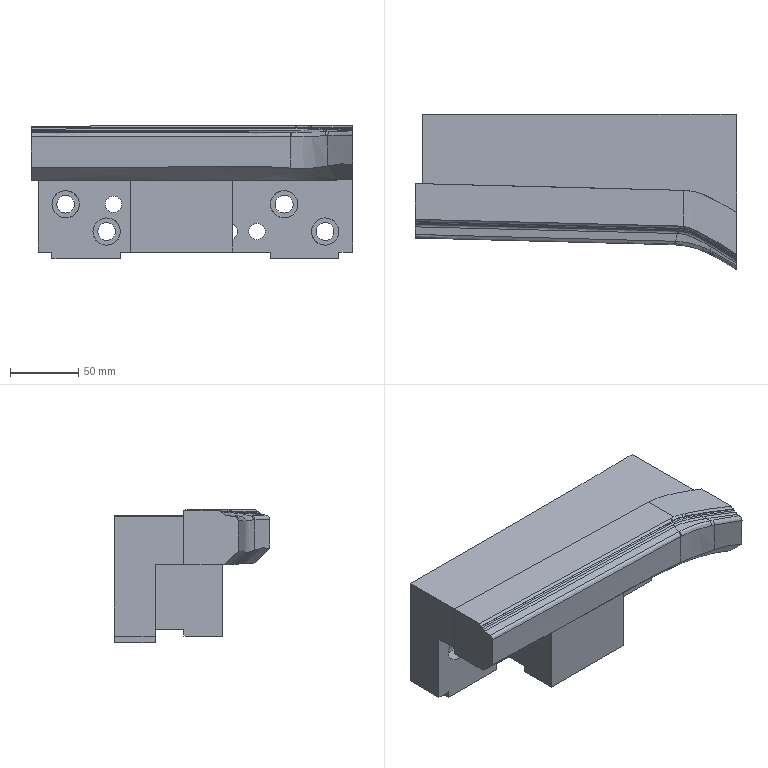Part | NX | features solid 2 | 1 solid | 77 faces | box 235 x 113.719 x 97.89 mm | volume 1323114 mm3 | spline 39 | plane 26 | cylinder 12 | commonest cylinder face diameters 12 x4 13 x4 20 x4